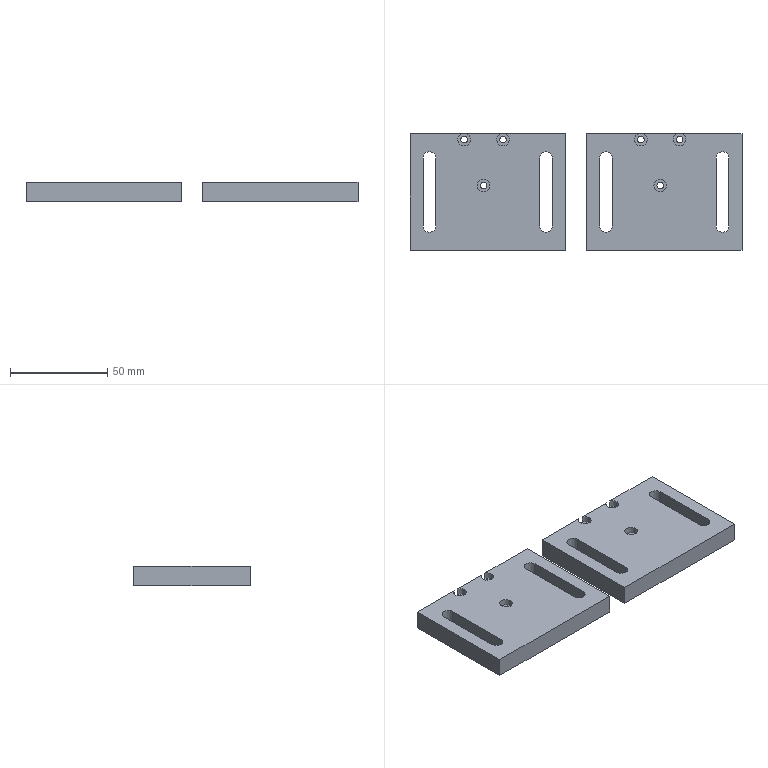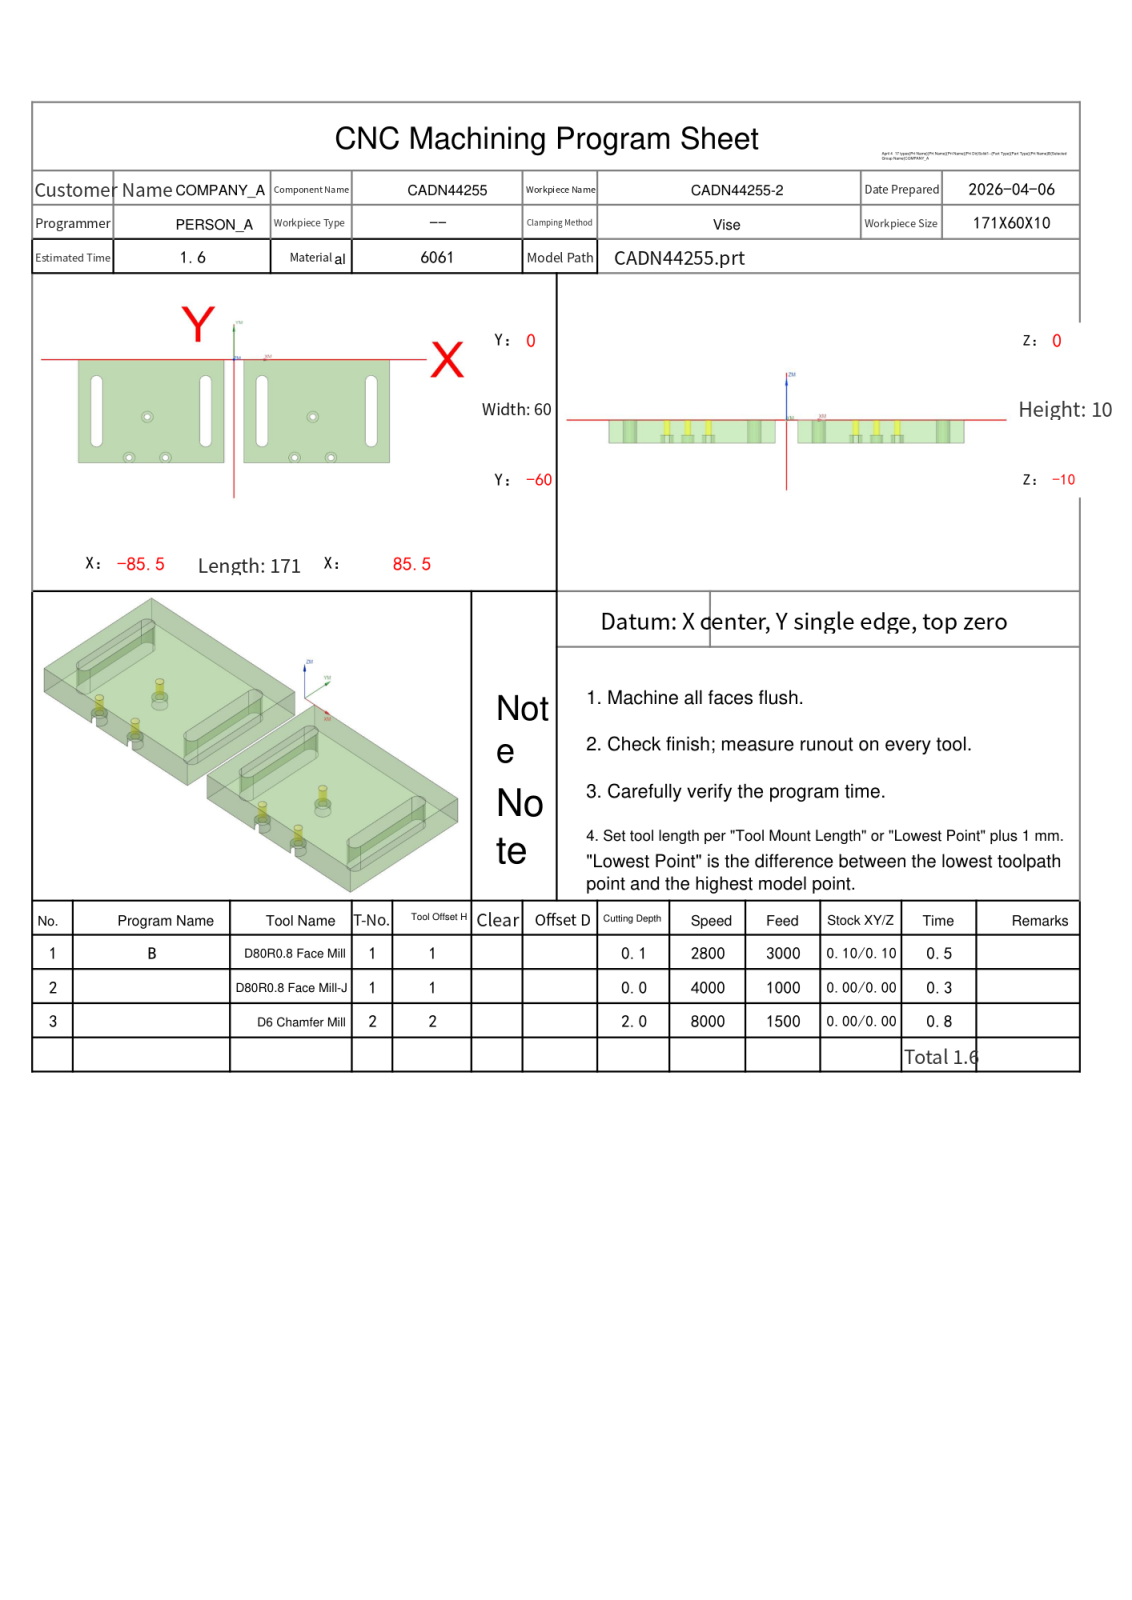NC program | NX | posted by the shop | part box 171 x 60 x 10 mm
Whole program:
%
O0001
(Machine time: 2.10 MIN)
(===Total Tool:2===)
(T1=D80R0.8 Face Mill D=80.  R=0.8  D-  H01 Z=0.    )
(T2=D6 Chamfer Mill  D=6.  R=0.  D-  H02 Z=-2.   )
G80 G90 G17 G49 G40
G91 G28 Z0
M01
N1 T01 M06
(D80R0.8 Face Mill  D=80. R=0.8 H=01 ce=0.10 di=0.10)
G00 G90 G54 X137.597 Y-30. M03 S2800
G43 H01 Z20.
M08
Z3.525
G01 Z1.525 F3000.
X125.597
X-125.597
X-137.597
Z3.525
G00 X137.597
Z3.05
G01 Z1.05
X125.597
X-125.597
X-137.597
Z3.05
G00 X137.597
Z2.575
G01 Z.575
X125.597
X-125.597
X-137.597
Z2.575
G00 X137.597
Z2.1
G01 Z.1
X125.597
X-125.597
X-137.597
Z2.1
G00 Z20.
G91 G28 Z0.0
M05
M09
G91 G28 Z0.0
M01
N2 T01 M06
(D80R0.8 Face Mill-J  D=80. R=0.8 H=01 ce=0.00 di=0.00)
G00 G90 G54 X137.499 Y-30. M03 S4000
G43 H01 Z20.
M08
Z2.
G01 Z0.0 F1000.
X125.499
X-125.499
X-137.499
Z2.
G00 Z20.
G91 G28 Z0.0
M05
M09
G91 G28 Z0.0
M01
N3 T02 M06
(D6 Chamfer Mill  D=6. R=0. H=02 ce=0.00 di=0.00)
G00 G90 G54 X43.393 Y-33.3 M03 S8000
G43 H02 Z20.
M08
G98 G81 X43.393 Y-33.3 Z-2. R3. F1000.
X53.393 Y-57.
X33.393
X-37.607
X-57.607
X-47.607 Y-33.3
G80
G00 Z20.
G00 G90 X45.114 Y1.227 M03 S6500
Z20.
Z.172
G01 Z-1.2 F1500.
G03 X45.4 Y1.027 I1.286 J1.532
G01 X45.446 Y.997
X45.5 Y1.
X85.5
G02 X86.5 Y0.0 I0.0 J-1.
G01 Y-60.
G02 X85.5 Y-61. I-1. J0.0
G01 X5.5
G02 X4.5 Y-60. I0.0 J1.
G01 Y0.0
G02 X5.5 Y1. I1. J0.0
G01 X45.5
X45.554 Y.997
X45.6 Y1.027
G03 X45.886 Y1.227 I-1. J1.732
G01 Z.172
G00 Z10.
X73.477 Y-29.614
Z.172
G01 Z-1.2
G03 X73.277 Y-29.9 I1.532 J-1.286
G01 X73.247 Y-29.946
X73.25 Y-30.
Y-47.5
G03 X75.5 Y-49.75 I2.25 J0.0
X77.75 Y-47.5 I0.0 J2.25
G01 Y-12.5
G03 X75.5 Y-10.25 I-2.25 J0.0
X73.25 Y-12.5 I0.0 J-2.25
G01 Y-30.
X73.247 Y-30.054
X73.277 Y-30.1
G03 X73.477 Y-30.386 I1.732 J1.
G01 Z.172
G00 Z10.
X52.868 Y-56.588
Z.376
G01 Z-1.2
G03 X52.707 Y-56.897 I1.687 J-1.075
G01 X52.684 Y-56.946
X52.693 Y-57.
G03 X53.393 Y-57.7 I.7 J0.0
X54.093 Y-57. I0.0 J.7
X53.393 Y-56.3 I-.7 J0.0
X52.717 Y-56.819 I0.0 J-.7
G01 X52.693 Y-57.
X52.684 Y-57.054
X52.707 Y-57.103
G03 X52.868 Y-57.412 I1.848 J.765
G01 Z.376
G00 Z10.
X32.868 Y-56.588
Z.376
G01 Z-1.2
G03 X32.707 Y-56.897 I1.687 J-1.075
G01 X32.684 Y-56.946
X32.693 Y-57.
G03 X33.393 Y-57.7 I.7 J0.0
X34.093 Y-57. I0.0 J.7
X33.393 Y-56.3 I-.7 J0.0
X32.717 Y-56.819 I0.0 J-.7
G01 X32.693 Y-57.
X32.684 Y-57.054
X32.707 Y-57.103
G03 X32.868 Y-57.412 I1.848 J.765
G01 Z.376
G00 Z10.
X42.868 Y-32.888
Z.376
G01 Z-1.2
G03 X42.707 Y-33.197 I1.687 J-1.075
G01 X42.684 Y-33.246
X42.693 Y-33.3
G03 X43.393 Y-34. I.7 J0.0
X44.093 Y-33.3 I0.0 J.7
X43.393 Y-32.6 I-.7 J0.0
X42.717 Y-33.119 I0.0 J-.7
G01 X42.693 Y-33.3
X42.684 Y-33.354
X42.707 Y-33.403
G03 X42.868 Y-33.712 I1.848 J.765
G01 Z.376
G00 Z10.
X13.477 Y-29.614
Z.172
G01 Z-1.2
G03 X13.277 Y-29.9 I1.532 J-1.286
G01 X13.247 Y-29.946
X13.25 Y-30.
Y-47.5
G03 X15.5 Y-49.75 I2.25 J0.0
X17.75 Y-47.5 I0.0 J2.25
G01 Y-12.5
G03 X15.5 Y-10.25 I-2.25 J0.0
X13.25 Y-12.5 I0.0 J-2.25
G01 Y-30.
X13.247 Y-30.054
X13.277 Y-30.1
G03 X13.477 Y-30.386 I1.732 J1.
G01 Z.172
G00 Z10.
X-45.886 Y1.227
Z.172
G01 Z-1.2
G03 X-45.6 Y1.027 I1.286 J1.532
G01 X-45.554 Y.997
X-45.5 Y1.
X-5.5
G02 X-4.5 Y0.0 I0.0 J-1.
G01 Y-60.
G02 X-5.5 Y-61. I-1. J0.0
G01 X-85.5
G02 X-86.5 Y-60. I0.0 J1.
G01 Y0.0
G02 X-85.5 Y1. I1. J0.0
G01 X-45.5
X-45.446 Y.997
X-45.4 Y1.027
G03 X-45.114 Y1.227 I-1. J1.732
G01 Z.172
G00 Z10.
X-17.523 Y-29.614
Z.172
G01 Z-1.2
G03 X-17.723 Y-29.9 I1.532 J-1.286
G01 X-17.753 Y-29.946
X-17.75 Y-30.
Y-47.5
G03 X-15.5 Y-49.75 I2.25 J0.0
X-13.25 Y-47.5 I0.0 J2.25
G01 Y-12.5
G03 X-15.5 Y-10.25 I-2.25 J0.0
X-17.75 Y-12.5 I0.0 J-2.25
G01 Y-30.
X-17.753 Y-30.054
X-17.723 Y-30.1
G03 X-17.523 Y-30.386 I1.732 J1.
G01 Z.172
G00 Z10.
X-38.132 Y-56.588
Z.376
G01 Z-1.2
G03 X-38.293 Y-56.897 I1.687 J-1.075
G01 X-38.316 Y-56.946
X-38.307 Y-57.
G03 X-37.607 Y-57.7 I.7 J0.0
X-36.907 Y-57. I0.0 J.7
X-37.607 Y-56.3 I-.7 J0.0
X-38.283 Y-56.819 I0.0 J-.7
G01 X-38.307 Y-57.
X-38.316 Y-57.054
X-38.293 Y-57.103
G03 X-38.132 Y-57.412 I1.848 J.765
G01 Z.376
G00 Z10.
X-58.132 Y-56.588
Z.376
G01 Z-1.2
G03 X-58.293 Y-56.897 I1.687 J-1.075
G01 X-58.316 Y-56.946
X-58.307 Y-57.
G03 X-57.607 Y-57.7 I.7 J0.0
X-56.907 Y-57. I0.0 J.7
X-57.607 Y-56.3 I-.7 J0.0
X-58.283 Y-56.819 I0.0 J-.7
G01 X-58.307 Y-57.
X-58.316 Y-57.054
X-58.293 Y-57.103
G03 X-58.132 Y-57.412 I1.848 J.765
G01 Z.376
G00 Z10.
X-48.132 Y-32.888
Z.376
G01 Z-1.2
G03 X-48.293 Y-33.197 I1.687 J-1.075
G01 X-48.316 Y-33.246
X-48.307 Y-33.3
G03 X-47.607 Y-34. I.7 J0.0
X-46.907 Y-33.3 I0.0 J.7
X-47.607 Y-32.6 I-.7 J0.0
X-48.283 Y-33.119 I0.0 J-.7
G01 X-48.307 Y-33.3
X-48.316 Y-33.354
X-48.293 Y-33.403
G03 X-48.132 Y-33.712 I1.848 J.765
G01 Z.376
G00 Z10.
X-73.477 Y-30.386
Z.172
G01 Z-1.2
G03 X-73.277 Y-30.1 I-1.532 J1.286
G01 X-73.247 Y-30.054
X-73.25 Y-30.
Y-12.5
G03 X-75.5 Y-10.25 I-2.25 J0.0
X-77.75 Y-12.5 I0.0 J-2.25
G01 Y-47.5
G03 X-75.5 Y-49.75 I2.25 J0.0
X-73.25 Y-47.5 I0.0 J2.25
G01 Y-30.
X-73.247 Y-29.946
X-73.277 Y-29.9
G03 X-73.477 Y-29.614 I-1.732 J-1.
G01 Z.172
G00 Z20.
M05
M09
G91 G28 Z0.0
G91 G28 Y0.0
M30
%